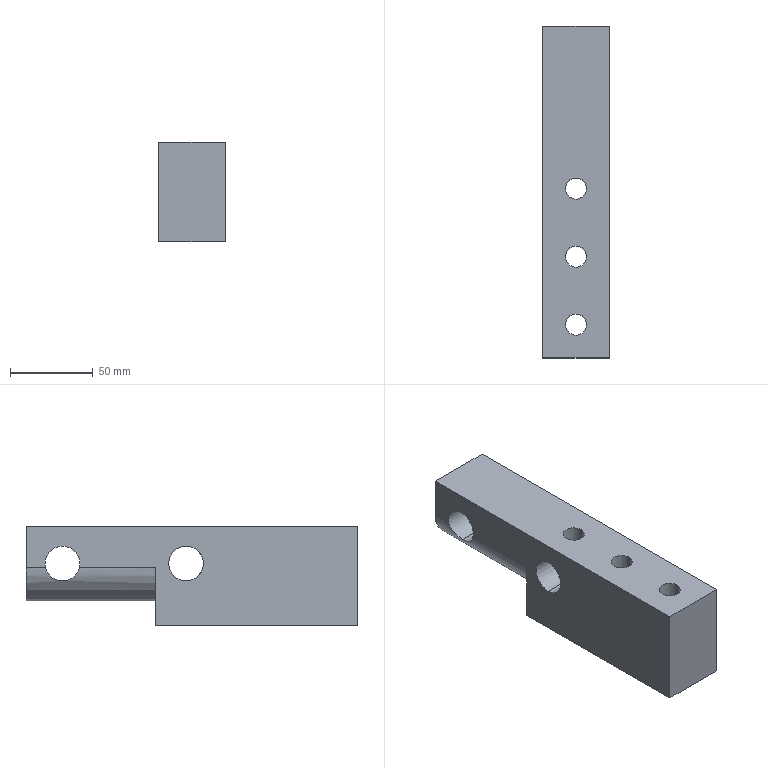Part | SolidWorks | features BaseBody 1 | 1 solid | 20 faces | box 40 x 200 x 60 mm | volume 371568 mm3 | cylinder 13 | plane 7 | commonest cylinder face diameters 12.8 x8 21 x4 40 x1
STEP:
#1=CARTESIAN_POINT('',(20.,67.862,5.));
#2=VERTEX_POINT('',#1);
#3=CARTESIAN_POINT('',(18.33,78.06,-3.));
#4=VERTEX_POINT('',#3);
#5=CARTESIAN_POINT('',(20.,67.862,5.));
#6=CARTESIAN_POINT('',(20.,68.003,4.424));
#7=CARTESIAN_POINT('',(19.975,68.191,3.869));
#8=CARTESIAN_POINT('',(19.886,68.653,2.8));
#9=CARTESIAN_POINT('',(19.821,68.929,2.283));
#10=CARTESIAN_POINT('',(19.661,69.566,1.299));
#11=CARTESIAN_POINT('',(19.568,69.921,0.8415));
#12=CARTESIAN_POINT('',(19.417,70.504,0.2031));
#13=CARTESIAN_POINT('',(19.366,70.708,-0.001681));
#14=CARTESIAN_POINT('',(19.26,71.132,-0.3951));
#15=CARTESIAN_POINT('',(19.205,71.354,-0.5846));
#16=CARTESIAN_POINT('',(19.044,72.039,-1.122));
#17=CARTESIAN_POINT('',(18.938,72.52,-1.438));
#18=CARTESIAN_POINT('',(18.79,73.278,-1.852));
#19=CARTESIAN_POINT('',(18.743,73.537,-1.98));
#20=CARTESIAN_POINT('',(18.653,74.068,-2.216));
#21=CARTESIAN_POINT('',(18.611,74.341,-2.324));
#22=CARTESIAN_POINT('',(18.496,75.171,-2.612));
#23=CARTESIAN_POINT('',(18.435,75.735,-2.756));
#24=CARTESIAN_POINT('',(18.352,76.882,-2.95));
#25=CARTESIAN_POINT('',(18.33,77.468,-3.));
#26=CARTESIAN_POINT('',(18.33,78.06,-3.));
#27=B_SPLINE_CURVE_WITH_KNOTS('',3,(#5,#6,#7,#8,#9,#10,#11,#12,#13,#14,#15,#16,#17,#18,#19,#20,#21,#22,#23,#24,#25,#26),.UNSPECIFIED.,.F.,.F.,(4,2,2,2,2,2,2,2,2,2,4),(0.,0.001752,0.003505,0.005257,0.006134,0.00701,0.008762,0.009639,0.01051,0.01227,0.01402),.UNSPECIFIED.);
#28=EDGE_CURVE('',#2,#4,#27,.T.);
#29=ORIENTED_EDGE('',*,*,#28,.T.);
#30=CARTESIAN_POINT('',(-18.33,78.06,-3.));
#31=VERTEX_POINT('',#30);
#32=CARTESIAN_POINT('',(58.,78.06,-3.));
#33=DIRECTION('',(-1.,0.,0.));
#34=VECTOR('',#33,1000.);
#35=LINE('',#32,#34);
#36=EDGE_CURVE('',#4,#31,#35,.T.);
#37=ORIENTED_EDGE('',*,*,#36,.T.);
#38=CARTESIAN_POINT('',(-20.,67.862,5.));
#39=VERTEX_POINT('',#38);
#40=CARTESIAN_POINT('',(-18.33,78.06,-3.));
#41=CARTESIAN_POINT('',(-18.33,77.469,-3.));
#42=CARTESIAN_POINT('',(-18.352,76.886,-2.95));
#43=CARTESIAN_POINT('',(-18.414,76.024,-2.805));
#44=CARTESIAN_POINT('',(-18.44,75.739,-2.744));
#45=CARTESIAN_POINT('',(-18.5,75.173,-2.6));
#46=CARTESIAN_POINT('',(-18.535,74.891,-2.515));
#47=CARTESIAN_POINT('',(-18.65,74.062,-2.227));
#48=CARTESIAN_POINT('',(-18.74,73.534,-1.992));
#49=CARTESIAN_POINT('',(-18.888,72.774,-1.577));
#50=CARTESIAN_POINT('',(-18.94,72.526,-1.428));
#51=CARTESIAN_POINT('',(-19.045,72.042,-1.109));
#52=CARTESIAN_POINT('',(-19.099,71.805,-0.9388));
#53=CARTESIAN_POINT('',(-19.26,71.123,-0.4035));
#54=CARTESIAN_POINT('',(-19.367,70.702,-0.01284));
#55=CARTESIAN_POINT('',(-19.517,70.119,0.6246));
#56=CARTESIAN_POINT('',(-19.565,69.933,0.8457));
#57=CARTESIAN_POINT('',(-19.657,69.577,1.306));
#58=CARTESIAN_POINT('',(-19.701,69.407,1.545));
#59=CARTESIAN_POINT('',(-19.82,68.931,2.279));
#60=CARTESIAN_POINT('',(-19.885,68.657,2.791));
#61=CARTESIAN_POINT('',(-19.975,68.193,3.862));
#62=CARTESIAN_POINT('',(-20.,68.003,4.424));
#63=CARTESIAN_POINT('',(-20.,67.862,5.));
#64=B_SPLINE_CURVE_WITH_KNOTS('',3,(#40,#41,#42,#43,#44,#45,#46,#47,#48,#49,#50,#51,#52,#53,#54,#55,#56,#57,#58,#59,#60,#61,#62,#63),.UNSPECIFIED.,.F.,.F.,(4,2,2,2,2,2,2,2,2,2,2,4),(0.01402,0.01577,0.01665,0.01752,0.01927,0.02015,0.02102,0.02277,0.02365,0.02452,0.02627,0.02802),.UNSPECIFIED.);
#65=EDGE_CURVE('',#31,#39,#64,.T.);
#66=ORIENTED_EDGE('',*,*,#65,.T.);
#67=CARTESIAN_POINT('',(-20.,78.06,18.));
#68=VERTEX_POINT('',#67);
#69=CARTESIAN_POINT('',(-20.,78.06,7.5));
#70=DIRECTION('',(-1.,0.,0.));
#71=DIRECTION('',(0.,0.,1.));
#72=AXIS2_PLACEMENT_3D('',#69,#70,#71);
#73=CIRCLE('',#72,10.5);
#74=EDGE_CURVE('',#39,#68,#73,.T.);
#75=ORIENTED_EDGE('',*,*,#74,.T.);
#76=CARTESIAN_POINT('',(20.,78.06,18.));
#77=VERTEX_POINT('',#76);
#78=CARTESIAN_POINT('',(58.,78.06,18.));
#79=DIRECTION('',(-1.,0.,0.));
#80=VECTOR('',#79,1000.);
#81=LINE('',#78,#80);
#82=EDGE_CURVE('',#77,#68,#81,.T.);
#83=ORIENTED_EDGE('',*,*,#82,.F.);
#84=CARTESIAN_POINT('',(20.,78.06,7.5));
#85=DIRECTION('',(-1.,0.,0.));
#86=DIRECTION('',(0.,0.,1.));
#87=AXIS2_PLACEMENT_3D('',#84,#85,#86);
#88=CIRCLE('',#87,10.5);
#89=EDGE_CURVE('',#2,#77,#88,.T.);
#90=ORIENTED_EDGE('',*,*,#89,.F.);
#91=EDGE_LOOP('',(#29,#37,#66,#75,#83,#90));
#92=FACE_OUTER_BOUND('',#91,.T.);
#93=CARTESIAN_POINT('',(58.,78.06,7.5));
#94=DIRECTION('',(-1.,0.,0.));
#95=DIRECTION('',(0.,0.,1.));
#96=AXIS2_PLACEMENT_3D('',#93,#94,#95);
#97=CYLINDRICAL_SURFACE('',#96,10.5);
#98=ADVANCED_FACE('',(#92),#97,.F.);
#99=CARTESIAN_POINT('',(20.,3.56,-3.));
#100=VERTEX_POINT('',#99);
#101=CARTESIAN_POINT('',(20.,3.56,18.));
#102=VERTEX_POINT('',#101);
#103=CARTESIAN_POINT('',(20.,3.56,7.5));
#104=DIRECTION('',(-1.,0.,0.));
#105=DIRECTION('',(0.,0.,1.));
#106=AXIS2_PLACEMENT_3D('',#103,#104,#105);
#107=CIRCLE('',#106,10.5);
#108=EDGE_CURVE('',#100,#102,#107,.T.);
#109=ORIENTED_EDGE('',*,*,#108,.F.);
#110=CARTESIAN_POINT('',(6.207,3.56,-3.));
#111=VERTEX_POINT('',#110);
#112=CARTESIAN_POINT('',(58.,3.56,-3.));
#113=DIRECTION('',(-1.,0.,0.));
#114=VECTOR('',#113,1000.);
#115=LINE('',#112,#114);
#116=EDGE_CURVE('',#100,#111,#115,.T.);
#117=ORIENTED_EDGE('',*,*,#116,.T.);
#118=CARTESIAN_POINT('',(6.4,2.,-2.883));
#119=VERTEX_POINT('',#118);
#120=CARTESIAN_POINT('',(6.4,2.,-2.883));
#121=CARTESIAN_POINT('',(6.4,2.259,-2.922));
#122=CARTESIAN_POINT('',(6.384,2.519,-2.952));
#123=CARTESIAN_POINT('',(6.32,3.04,-2.99));
#124=CARTESIAN_POINT('',(6.271,3.304,-3.));
#125=CARTESIAN_POINT('',(6.207,3.56,-3.));
#126=B_SPLINE_CURVE_WITH_KNOTS('',3,(#120,#121,#122,#123,#124,#125),.UNSPECIFIED.,.F.,.F.,(4,2,4),(0.02134,0.02212,0.02291),.UNSPECIFIED.);
#127=EDGE_CURVE('',#119,#111,#126,.T.);
#128=ORIENTED_EDGE('',*,*,#127,.F.);
#129=CARTESIAN_POINT('',(-6.4,2.,-2.883));
#130=VERTEX_POINT('',#129);
#131=CARTESIAN_POINT('',(-6.4,2.,-2.883));
#132=CARTESIAN_POINT('',(-6.4,1.553,-2.816));
#133=CARTESIAN_POINT('',(-6.354,1.12,-2.722));
#134=CARTESIAN_POINT('',(-6.18,0.2803,-2.484));
#135=CARTESIAN_POINT('',(-6.049,-0.1306,-2.339));
#136=CARTESIAN_POINT('',(-5.722,-0.897,-2.016));
#137=CARTESIAN_POINT('',(-5.525,-1.256,-1.839));
#138=CARTESIAN_POINT('',(-5.067,-1.93,-1.459));
#139=CARTESIAN_POINT('',(-4.811,-2.24,-1.26));
#140=CARTESIAN_POINT('',(-4.388,-2.663,-0.9592));
#141=CARTESIAN_POINT('',(-4.241,-2.797,-0.8585));
#142=CARTESIAN_POINT('',(-3.933,-3.053,-0.6579));
#143=CARTESIAN_POINT('',(-3.772,-3.174,-0.5574));
#144=CARTESIAN_POINT('',(-3.272,-3.515,-0.2639));
#145=CARTESIAN_POINT('',(-2.917,-3.712,-0.07815));
#146=CARTESIAN_POINT('',(-2.155,-4.04,0.2517));
#147=CARTESIAN_POINT('',(-1.744,-4.173,0.3961));
#148=CARTESIAN_POINT('',(-1.105,-4.308,0.5463));
#149=CARTESIAN_POINT('',(-0.8875,-4.342,0.5857));
#150=CARTESIAN_POINT('',(-0.4424,-4.389,0.6392));
#151=CARTESIAN_POINT('',(-0.2165,-4.4,0.6528));
#152=CARTESIAN_POINT('',(0.2295,-4.4,0.6522));
#153=CARTESIAN_POINT('',(0.4515,-4.388,0.6384));
#154=CARTESIAN_POINT('',(0.8932,-4.341,0.5847));
#155=CARTESIAN_POINT('',(1.115,-4.306,0.5444));
#156=CARTESIAN_POINT('',(1.756,-4.17,0.3926));
#157=CARTESIAN_POINT('',(2.158,-4.04,0.2509));
#158=CARTESIAN_POINT('',(2.925,-3.708,-0.08206));
#159=CARTESIAN_POINT('',(3.281,-3.509,-0.2694));
#160=CARTESIAN_POINT('',(3.942,-3.058,-0.6575));
#161=CARTESIAN_POINT('',(4.249,-2.803,-0.8599));
#162=CARTESIAN_POINT('',(4.816,-2.234,-1.264));
#163=CARTESIAN_POINT('',(5.07,-1.926,-1.461));
#164=CARTESIAN_POINT('',(5.41,-1.426,-1.743));
#165=CARTESIAN_POINT('',(5.515,-1.253,-1.834));
#166=CARTESIAN_POINT('',(5.712,-0.893,-2.011));
#167=CARTESIAN_POINT('',(5.804,-0.705,-2.097));
#168=CARTESIAN_POINT('',(6.051,-0.1275,-2.34));
#169=CARTESIAN_POINT('',(6.178,0.2748,-2.482));
#170=CARTESIAN_POINT('',(6.31,0.907,-2.662));
#171=CARTESIAN_POINT('',(6.344,1.124,-2.716));
#172=CARTESIAN_POINT('',(6.389,1.561,-2.81));
#173=CARTESIAN_POINT('',(6.4,1.78,-2.85));
#174=CARTESIAN_POINT('',(6.4,2.,-2.883));
#175=B_SPLINE_CURVE_WITH_KNOTS('',3,(#131,#132,#133,#134,#135,#136,#137,#138,#139,#140,#141,#142,#143,#144,#145,#146,#147,#148,#149,#150,#151,#152,#153,#154,#155,#156,#157,#158,#159,#160,#161,#162,#163,#164,#165,#166,#167,#168,#169,#170,#171,#172,#173,#174),.UNSPECIFIED.,.F.,.F.,(4,2,2,2,2,2,2,2,2,2,2,2,2,2,2,2,2,2,2,2,2,4),(0.,0.001334,0.002667,0.004001,0.005334,0.006001,0.006668,0.008001,0.009335,0.01,0.01067,0.01134,0.012,0.01334,0.01467,0.016,0.01734,0.018,0.01867,0.02,0.02067,0.02134),.UNSPECIFIED.);
#176=EDGE_CURVE('',#130,#119,#175,.T.);
#177=ORIENTED_EDGE('',*,*,#176,.F.);
#178=CARTESIAN_POINT('',(-6.207,3.56,-3.));
#179=VERTEX_POINT('',#178);
#180=CARTESIAN_POINT('',(-6.207,3.56,-3.));
#181=CARTESIAN_POINT('',(-6.271,3.307,-3.));
#182=CARTESIAN_POINT('',(-6.319,3.05,-2.991));
#183=CARTESIAN_POINT('',(-6.384,2.528,-2.952));
#184=CARTESIAN_POINT('',(-6.4,2.263,-2.923));
#185=CARTESIAN_POINT('',(-6.4,2.,-2.883));
#186=B_SPLINE_CURVE_WITH_KNOTS('',3,(#180,#181,#182,#183,#184,#185),.UNSPECIFIED.,.F.,.F.,(4,2,4),(0.03996,0.04074,0.04152),.UNSPECIFIED.);
#187=EDGE_CURVE('',#179,#130,#186,.T.);
#188=ORIENTED_EDGE('',*,*,#187,.F.);
#189=CARTESIAN_POINT('',(-20.,3.56,-3.));
#190=VERTEX_POINT('',#189);
#191=CARTESIAN_POINT('',(58.,3.56,-3.));
#192=DIRECTION('',(-1.,0.,0.));
#193=VECTOR('',#192,1000.);
#194=LINE('',#191,#193);
#195=EDGE_CURVE('',#179,#190,#194,.T.);
#196=ORIENTED_EDGE('',*,*,#195,.T.);
#197=CARTESIAN_POINT('',(-20.,3.56,18.));
#198=VERTEX_POINT('',#197);
#199=CARTESIAN_POINT('',(-20.,3.56,7.5));
#200=DIRECTION('',(-1.,0.,0.));
#201=DIRECTION('',(0.,0.,1.));
#202=AXIS2_PLACEMENT_3D('',#199,#200,#201);
#203=CIRCLE('',#202,10.5);
#204=EDGE_CURVE('',#190,#198,#203,.T.);
#205=ORIENTED_EDGE('',*,*,#204,.T.);
#206=CARTESIAN_POINT('',(-6.207,3.56,18.));
#207=VERTEX_POINT('',#206);
#208=CARTESIAN_POINT('',(58.,3.56,18.));
#209=DIRECTION('',(-1.,0.,0.));
#210=VECTOR('',#209,1000.);
#211=LINE('',#208,#210);
#212=EDGE_CURVE('',#207,#198,#211,.T.);
#213=ORIENTED_EDGE('',*,*,#212,.F.);
#214=CARTESIAN_POINT('',(-6.4,2.,17.883));
#215=VERTEX_POINT('',#214);
#216=CARTESIAN_POINT('',(-6.4,2.,17.883));
#217=CARTESIAN_POINT('',(-6.4,2.264,17.923));
#218=CARTESIAN_POINT('',(-6.384,2.525,17.952));
#219=CARTESIAN_POINT('',(-6.319,3.045,17.991));
#220=CARTESIAN_POINT('',(-6.271,3.304,18.));
#221=CARTESIAN_POINT('',(-6.207,3.56,18.));
#222=B_SPLINE_CURVE_WITH_KNOTS('',3,(#216,#217,#218,#219,#220,#221),.UNSPECIFIED.,.F.,.F.,(4,2,4),(0.,0.0007878,0.001576),.UNSPECIFIED.);
#223=EDGE_CURVE('',#215,#207,#222,.T.);
#224=ORIENTED_EDGE('',*,*,#223,.F.);
#225=CARTESIAN_POINT('',(6.4,2.,17.883));
#226=VERTEX_POINT('',#225);
#227=CARTESIAN_POINT('',(6.4,2.,17.883));
#228=CARTESIAN_POINT('',(6.4,1.778,17.85));
#229=CARTESIAN_POINT('',(6.388,1.556,17.809));
#230=CARTESIAN_POINT('',(6.343,1.121,17.715));
#231=CARTESIAN_POINT('',(6.31,0.9071,17.662));
#232=CARTESIAN_POINT('',(6.178,0.2763,17.483));
#233=CARTESIAN_POINT('',(6.048,-0.134,17.338));
#234=CARTESIAN_POINT('',(5.72,-0.9001,17.015));
#235=CARTESIAN_POINT('',(5.523,-1.259,16.837));
#236=CARTESIAN_POINT('',(5.065,-1.933,16.457));
#237=CARTESIAN_POINT('',(4.809,-2.242,16.258));
#238=CARTESIAN_POINT('',(4.387,-2.664,15.958));
#239=CARTESIAN_POINT('',(4.24,-2.798,15.857));
#240=CARTESIAN_POINT('',(3.932,-3.054,15.657));
#241=CARTESIAN_POINT('',(3.77,-3.176,15.556));
#242=CARTESIAN_POINT('',(3.27,-3.516,15.263));
#243=CARTESIAN_POINT('',(2.916,-3.712,15.078));
#244=CARTESIAN_POINT('',(2.155,-4.041,14.748));
#245=CARTESIAN_POINT('',(1.743,-4.173,14.604));
#246=CARTESIAN_POINT('',(1.105,-4.308,14.454));
#247=CARTESIAN_POINT('',(0.8875,-4.342,14.414));
#248=CARTESIAN_POINT('',(0.4424,-4.389,14.361));
#249=CARTESIAN_POINT('',(0.217,-4.4,14.347));
#250=CARTESIAN_POINT('',(-0.2285,-4.4,14.348));
#251=CARTESIAN_POINT('',(-0.4503,-4.388,14.362));
#252=CARTESIAN_POINT('',(-0.892,-4.341,14.415));
#253=CARTESIAN_POINT('',(-1.113,-4.306,14.455));
#254=CARTESIAN_POINT('',(-1.754,-4.171,14.607));
#255=CARTESIAN_POINT('',(-2.156,-4.04,14.748));
#256=CARTESIAN_POINT('',(-2.924,-3.708,15.081));
#257=CARTESIAN_POINT('',(-3.279,-3.511,15.268));
#258=CARTESIAN_POINT('',(-3.939,-3.06,15.656));
#259=CARTESIAN_POINT('',(-4.247,-2.804,15.859));
#260=CARTESIAN_POINT('',(-4.814,-2.237,16.262));
#261=CARTESIAN_POINT('',(-5.068,-1.929,16.459));
#262=CARTESIAN_POINT('',(-5.407,-1.43,16.741));
#263=CARTESIAN_POINT('',(-5.513,-1.257,16.832));
#264=CARTESIAN_POINT('',(-5.71,-0.8971,17.009));
#265=CARTESIAN_POINT('',(-5.802,-0.7091,17.095));
#266=CARTESIAN_POINT('',(-6.049,-0.1327,17.338));
#267=CARTESIAN_POINT('',(-6.176,0.2691,17.481));
#268=CARTESIAN_POINT('',(-6.353,1.112,17.72));
#269=CARTESIAN_POINT('',(-6.4,1.554,17.816));
#270=CARTESIAN_POINT('',(-6.4,2.,17.883));
#271=B_SPLINE_CURVE_WITH_KNOTS('',3,(#227,#228,#229,#230,#231,#232,#233,#234,#235,#236,#237,#238,#239,#240,#241,#242,#243,#244,#245,#246,#247,#248,#249,#250,#251,#252,#253,#254,#255,#256,#257,#258,#259,#260,#261,#262,#263,#264,#265,#266,#267,#268,#269,#270),.UNSPECIFIED.,.F.,.F.,(4,2,2,2,2,2,2,2,2,2,2,2,2,2,2,2,2,2,2,2,2,4),(0.02022,0.02089,0.02156,0.02289,0.02422,0.02555,0.02622,0.02689,0.02822,0.02955,0.03022,0.03089,0.03155,0.03222,0.03355,0.03488,0.03622,0.03755,0.03822,0.03888,0.04022,0.04155),.UNSPECIFIED.);
#272=EDGE_CURVE('',#226,#215,#271,.T.);
#273=ORIENTED_EDGE('',*,*,#272,.F.);
#274=CARTESIAN_POINT('',(6.207,3.56,18.));
#275=VERTEX_POINT('',#274);
#276=CARTESIAN_POINT('',(6.207,3.56,18.));
#277=CARTESIAN_POINT('',(6.272,3.302,18.));
#278=CARTESIAN_POINT('',(6.32,3.043,17.991));
#279=CARTESIAN_POINT('',(6.384,2.523,17.952));
#280=CARTESIAN_POINT('',(6.4,2.262,17.923));
#281=CARTESIAN_POINT('',(6.4,2.,17.883));
#282=B_SPLINE_CURVE_WITH_KNOTS('',3,(#276,#277,#278,#279,#280,#281),.UNSPECIFIED.,.F.,.F.,(4,2,4),(0.01865,0.01943,0.02022),.UNSPECIFIED.);
#283=EDGE_CURVE('',#275,#226,#282,.T.);
#284=ORIENTED_EDGE('',*,*,#283,.F.);
#285=CARTESIAN_POINT('',(58.,3.56,18.));
#286=DIRECTION('',(-1.,0.,0.));
#287=VECTOR('',#286,1000.);
#288=LINE('',#285,#287);
#289=EDGE_CURVE('',#102,#275,#288,.T.);
#290=ORIENTED_EDGE('',*,*,#289,.F.);
#291=EDGE_LOOP('',(#109,#117,#128,#177,#188,#196,#205,#213,#224,#273,#284,#290));
#292=FACE_OUTER_BOUND('',#291,.T.);
#293=CARTESIAN_POINT('',(58.,3.56,7.5));
#294=DIRECTION('',(-1.,0.,0.));
#295=DIRECTION('',(0.,0.,1.));
#296=AXIS2_PLACEMENT_3D('',#293,#294,#295);
#297=CYLINDRICAL_SURFACE('',#296,10.5);
#298=ADVANCED_FACE('',(#292),#297,.F.);
#299=ORIENTED_EDGE('',*,*,#176,.T.);
#300=CARTESIAN_POINT('',(6.4,2.,-30.));
#301=VERTEX_POINT('',#300);
#302=CARTESIAN_POINT('',(6.4,2.,48.));
#303=DIRECTION('',(0.,0.,-1.));
#304=VECTOR('',#303,1000.);
#305=LINE('',#302,#304);
#306=EDGE_CURVE('',#119,#301,#305,.T.);
#307=ORIENTED_EDGE('',*,*,#306,.T.);
#308=CARTESIAN_POINT('',(-6.4,2.,-30.));
#309=VERTEX_POINT('',#308);
#310=CARTESIAN_POINT('',(0.,2.,-30.));
#311=DIRECTION('',(0.,0.,-1.));
#312=DIRECTION('',(1.,0.,0.));
#313=AXIS2_PLACEMENT_3D('',#310,#311,#312);
#314=CIRCLE('',#313,6.4);
#315=EDGE_CURVE('',#301,#309,#314,.T.);
#316=ORIENTED_EDGE('',*,*,#315,.T.);
#317=CARTESIAN_POINT('',(-6.4,2.,48.));
#318=DIRECTION('',(0.,0.,-1.));
#319=VECTOR('',#318,1000.);
#320=LINE('',#317,#319);
#321=EDGE_CURVE('',#130,#309,#320,.T.);
#322=ORIENTED_EDGE('',*,*,#321,.F.);
#323=EDGE_LOOP('',(#299,#307,#316,#322));
#324=FACE_OUTER_BOUND('',#323,.T.);
#325=CARTESIAN_POINT('',(0.,2.,48.));
#326=DIRECTION('',(0.,0.,-1.));
#327=DIRECTION('',(-1.,0.,0.));
#328=AXIS2_PLACEMENT_3D('',#325,#326,#327);
#329=CYLINDRICAL_SURFACE('',#328,6.4);
#330=ADVANCED_FACE('',(#324),#329,.F.);
#331=CARTESIAN_POINT('',(6.4,-80.,30.));
#332=VERTEX_POINT('',#331);
#333=CARTESIAN_POINT('',(-6.4,-80.,30.));
#334=VERTEX_POINT('',#333);
#335=CARTESIAN_POINT('',(0.,-80.,30.));
#336=DIRECTION('',(0.,0.,-1.));
#337=DIRECTION('',(-1.,0.,0.));
#338=AXIS2_PLACEMENT_3D('',#335,#336,#337);
#339=CIRCLE('',#338,6.4);
#340=EDGE_CURVE('',#332,#334,#339,.T.);
#341=ORIENTED_EDGE('',*,*,#340,.F.);
#342=CARTESIAN_POINT('',(6.4,-80.,-30.));
#343=VERTEX_POINT('',#342);
#344=CARTESIAN_POINT('',(6.4,-80.,48.));
#345=DIRECTION('',(0.,0.,-1.));
#346=VECTOR('',#345,1000.);
#347=LINE('',#344,#346);
#348=EDGE_CURVE('',#332,#343,#347,.T.);
#349=ORIENTED_EDGE('',*,*,#348,.T.);
#350=CARTESIAN_POINT('',(-6.4,-80.,-30.));
#351=VERTEX_POINT('',#350);
#352=CARTESIAN_POINT('',(0.,-80.,-30.));
#353=DIRECTION('',(0.,0.,-1.));
#354=DIRECTION('',(-1.,0.,0.));
#355=AXIS2_PLACEMENT_3D('',#352,#353,#354);
#356=CIRCLE('',#355,6.4);
#357=EDGE_CURVE('',#343,#351,#356,.T.);
#358=ORIENTED_EDGE('',*,*,#357,.T.);
#359=CARTESIAN_POINT('',(-6.4,-80.,48.));
#360=DIRECTION('',(0.,0.,-1.));
#361=VECTOR('',#360,1000.);
#362=LINE('',#359,#361);
#363=EDGE_CURVE('',#334,#351,#362,.T.);
#364=ORIENTED_EDGE('',*,*,#363,.F.);
#365=EDGE_LOOP('',(#341,#349,#358,#364));
#366=FACE_OUTER_BOUND('',#365,.T.);
#367=CARTESIAN_POINT('',(0.,-80.,48.));
#368=DIRECTION('',(0.,0.,-1.));
#369=DIRECTION('',(-1.,0.,0.));
#370=AXIS2_PLACEMENT_3D('',#367,#368,#369);
#371=CYLINDRICAL_SURFACE('',#370,6.4);
#372=ADVANCED_FACE('',(#366),#371,.F.);
#373=CARTESIAN_POINT('',(6.4,-39.,30.));
#374=VERTEX_POINT('',#373);
#375=CARTESIAN_POINT('',(-6.4,-39.,30.));
#376=VERTEX_POINT('',#375);
#377=CARTESIAN_POINT('',(0.,-39.,30.));
#378=DIRECTION('',(0.,0.,-1.));
#379=DIRECTION('',(-1.,0.,0.));
#380=AXIS2_PLACEMENT_3D('',#377,#378,#379);
#381=CIRCLE('',#380,6.4);
#382=EDGE_CURVE('',#374,#376,#381,.T.);
#383=ORIENTED_EDGE('',*,*,#382,.F.);
#384=CARTESIAN_POINT('',(6.4,-39.,-30.));
#385=VERTEX_POINT('',#384);
#386=CARTESIAN_POINT('',(6.4,-39.,48.));
#387=DIRECTION('',(0.,0.,-1.));
#388=VECTOR('',#387,1000.);
#389=LINE('',#386,#388);
#390=EDGE_CURVE('',#374,#385,#389,.T.);
#391=ORIENTED_EDGE('',*,*,#390,.T.);
#392=CARTESIAN_POINT('',(-6.4,-39.,-30.));
#393=VERTEX_POINT('',#392);
#394=CARTESIAN_POINT('',(0.,-39.,-30.));
#395=DIRECTION('',(0.,0.,-1.));
#396=DIRECTION('',(-1.,0.,0.));
#397=AXIS2_PLACEMENT_3D('',#394,#395,#396);
#398=CIRCLE('',#397,6.4);
#399=EDGE_CURVE('',#385,#393,#398,.T.);
#400=ORIENTED_EDGE('',*,*,#399,.T.);
#401=CARTESIAN_POINT('',(-6.4,-39.,48.));
#402=DIRECTION('',(0.,0.,-1.));
#403=VECTOR('',#402,1000.);
#404=LINE('',#401,#403);
#405=EDGE_CURVE('',#376,#393,#404,.T.);
#406=ORIENTED_EDGE('',*,*,#405,.F.);
#407=EDGE_LOOP('',(#383,#391,#400,#406));
#408=FACE_OUTER_BOUND('',#407,.T.);
#409=CARTESIAN_POINT('',(0.,-39.,48.));
#410=DIRECTION('',(0.,0.,-1.));
#411=DIRECTION('',(-1.,0.,0.));
#412=AXIS2_PLACEMENT_3D('',#409,#410,#411);
#413=CYLINDRICAL_SURFACE('',#412,6.4);
#414=ADVANCED_FACE('',(#408),#413,.F.);
#415=CARTESIAN_POINT('',(6.4,2.,30.));
#416=VERTEX_POINT('',#415);
#417=CARTESIAN_POINT('',(-6.4,2.,30.));
#418=VERTEX_POINT('',#417);
#419=CARTESIAN_POINT('',(0.,2.,30.));
#420=DIRECTION('',(0.,0.,-1.));
#421=DIRECTION('',(-1.,0.,0.));
#422=AXIS2_PLACEMENT_3D('',#419,#420,#421);
#423=CIRCLE('',#422,6.4);
#424=EDGE_CURVE('',#416,#418,#423,.T.);
#425=ORIENTED_EDGE('',*,*,#424,.F.);
#426=CARTESIAN_POINT('',(6.4,2.,48.));
#427=DIRECTION('',(0.,0.,-1.));
#428=VECTOR('',#427,1000.);
#429=LINE('',#426,#428);
#430=EDGE_CURVE('',#416,#226,#429,.T.);
#431=ORIENTED_EDGE('',*,*,#430,.T.);
#432=ORIENTED_EDGE('',*,*,#272,.T.);
#433=CARTESIAN_POINT('',(-6.4,2.,48.));
#434=DIRECTION('',(0.,0.,-1.));
#435=VECTOR('',#434,1000.);
#436=LINE('',#433,#435);
#437=EDGE_CURVE('',#418,#215,#436,.T.);
#438=ORIENTED_EDGE('',*,*,#437,.F.);
#439=EDGE_LOOP('',(#425,#431,#432,#438));
#440=FACE_OUTER_BOUND('',#439,.T.);
#441=CARTESIAN_POINT('',(0.,2.,48.));
#442=DIRECTION('',(0.,0.,-1.));
#443=DIRECTION('',(-1.,0.,0.));
#444=AXIS2_PLACEMENT_3D('',#441,#442,#443);
#445=CYLINDRICAL_SURFACE('',#444,6.4);
#446=ADVANCED_FACE('',(#440),#445,.F.);
#447=ORIENTED_EDGE('',*,*,#430,.F.);
#448=CARTESIAN_POINT('',(0.,2.,30.));
#449=DIRECTION('',(0.,0.,-1.));
#450=DIRECTION('',(-1.,0.,0.));
#451=AXIS2_PLACEMENT_3D('',#448,#449,#450);
#452=CIRCLE('',#451,6.4);
#453=EDGE_CURVE('',#418,#416,#452,.T.);
#454=ORIENTED_EDGE('',*,*,#453,.F.);
#455=ORIENTED_EDGE('',*,*,#437,.T.);
#456=ORIENTED_EDGE('',*,*,#223,.T.);
#457=CARTESIAN_POINT('',(-6.207,3.56,18.));
#458=CARTESIAN_POINT('',(-6.163,3.734,18.));
#459=CARTESIAN_POINT('',(-6.112,3.907,17.996));
#460=CARTESIAN_POINT('',(-5.996,4.246,17.979));
#461=CARTESIAN_POINT('',(-5.931,4.412,17.967));
#462=CARTESIAN_POINT('',(-5.716,4.9,17.919));
#463=CARTESIAN_POINT('',(-5.548,5.211,17.874));
#464=CARTESIAN_POINT('',(-4.963,6.103,17.705));
#465=CARTESIAN_POINT('',(-4.486,6.618,17.555));
#466=CARTESIAN_POINT('',(-3.377,7.482,17.251));
#467=CARTESIAN_POINT('',(-2.765,7.816,17.102));
#468=CARTESIAN_POINT('',(-1.419,8.281,16.882));
#469=CARTESIAN_POINT('',(-0.7225,8.4,16.818));
#470=CARTESIAN_POINT('',(0.3589,8.4,16.818));
#471=CARTESIAN_POINT('',(0.7155,8.37,16.834));
#472=CARTESIAN_POINT('',(1.415,8.252,16.894));
#473=CARTESIAN_POINT('',(1.76,8.163,16.938));
#474=CARTESIAN_POINT('',(2.432,7.93,17.048));
#475=CARTESIAN_POINT('',(2.753,7.788,17.113));
#476=CARTESIAN_POINT('',(3.367,7.454,17.253));
#477=CARTESIAN_POINT('',(3.663,7.26,17.329));
#478=CARTESIAN_POINT('',(4.215,6.829,17.481));
#479=CARTESIAN_POINT('',(4.471,6.593,17.556));
#480=CARTESIAN_POINT('',(4.826,6.207,17.662));
#481=CARTESIAN_POINT('',(4.939,6.074,17.696));
#482=CARTESIAN_POINT('',(5.156,5.796,17.76));
#483=CARTESIAN_POINT('',(5.26,5.651,17.791));
#484=CARTESIAN_POINT('',(5.55,5.206,17.875));
#485=CARTESIAN_POINT('',(5.718,4.896,17.92));
#486=CARTESIAN_POINT('',(5.931,4.411,17.967));
#487=CARTESIAN_POINT('',(5.996,4.246,17.979));
#488=CARTESIAN_POINT('',(6.112,3.908,17.996));
#489=CARTESIAN_POINT('',(6.163,3.734,18.));
#490=CARTESIAN_POINT('',(6.207,3.56,18.));
#491=B_SPLINE_CURVE_WITH_KNOTS('',3,(#457,#458,#459,#460,#461,#462,#463,#464,#465,#466,#467,#468,#469,#470,#471,#472,#473,#474,#475,#476,#477,#478,#479,#480,#481,#482,#483,#484,#485,#486,#487,#488,#489,#490),.UNSPECIFIED.,.F.,.F.,(4,2,2,2,2,2,2,2,2,2,2,2,2,2,2,2,4),(0.001576,0.002109,0.002642,0.003709,0.005843,0.007977,0.01011,0.01118,0.01224,0.01331,0.01438,0.01544,0.01598,0.01651,0.01758,0.01811,0.01865),.UNSPECIFIED.);
#492=EDGE_CURVE('',#207,#275,#491,.T.);
#493=ORIENTED_EDGE('',*,*,#492,.T.);
#494=ORIENTED_EDGE('',*,*,#283,.T.);
#495=EDGE_LOOP('',(#447,#454,#455,#456,#493,#494));
#496=FACE_OUTER_BOUND('',#495,.T.);
#497=CARTESIAN_POINT('',(0.,2.,48.));
#498=DIRECTION('',(0.,0.,-1.));
#499=DIRECTION('',(-1.,0.,0.));
#500=AXIS2_PLACEMENT_3D('',#497,#498,#499);
#501=CYLINDRICAL_SURFACE('',#500,6.4);
#502=ADVANCED_FACE('',(#496),#501,.F.);
#503=CARTESIAN_POINT('',(0.,2.,-30.));
#504=DIRECTION('',(0.,0.,-1.));
#505=DIRECTION('',(1.,0.,0.));
#506=AXIS2_PLACEMENT_3D('',#503,#504,#505);
#507=CIRCLE('',#506,6.4);
#508=EDGE_CURVE('',#309,#301,#507,.T.);
#509=ORIENTED_EDGE('',*,*,#508,.F.);
#510=ORIENTED_EDGE('',*,*,#315,.F.);
#511=EDGE_LOOP('',(#509,#510));
#512=FACE_BOUND('',#511,.T.);
#513=CARTESIAN_POINT('',(0.,-80.,-30.));
#514=DIRECTION('',(0.,0.,-1.));
#515=DIRECTION('',(-1.,0.,0.));
#516=AXIS2_PLACEMENT_3D('',#513,#514,#515);
#517=CIRCLE('',#516,6.4);
#518=EDGE_CURVE('',#351,#343,#517,.T.);
#519=ORIENTED_EDGE('',*,*,#518,.F.);
#520=ORIENTED_EDGE('',*,*,#357,.F.);
#521=EDGE_LOOP('',(#519,#520));
#522=FACE_BOUND('',#521,.T.);
#523=CARTESIAN_POINT('',(0.,-39.,-30.));
#524=DIRECTION('',(0.,0.,-1.));
#525=DIRECTION('',(-1.,0.,0.));
#526=AXIS2_PLACEMENT_3D('',#523,#524,#525);
#527=CIRCLE('',#526,6.4);
#528=EDGE_CURVE('',#393,#385,#527,.T.);
#529=ORIENTED_EDGE('',*,*,#528,.F.);
#530=ORIENTED_EDGE('',*,*,#399,.F.);
#531=EDGE_LOOP('',(#529,#530));
#532=FACE_BOUND('',#531,.T.);
#533=CARTESIAN_POINT('',(20.,22.,-30.));
#534=VERTEX_POINT('',#533);
#535=CARTESIAN_POINT('',(-20.,22.,-30.));
#536=VERTEX_POINT('',#535);
#537=CARTESIAN_POINT('',(0.,22.,-30.));
#538=DIRECTION('',(-1.,0.,0.));
#539=VECTOR('',#538,1000.);
#540=LINE('',#537,#539);
#541=EDGE_CURVE('',#534,#536,#540,.T.);
#542=ORIENTED_EDGE('',*,*,#541,.F.);
#543=CARTESIAN_POINT('',(20.,-100.,-30.));
#544=VERTEX_POINT('',#543);
#545=CARTESIAN_POINT('',(20.,100.,-30.));
#546=DIRECTION('',(0.,-1.,0.));
#547=VECTOR('',#546,1000.);
#548=LINE('',#545,#547);
#549=EDGE_CURVE('',#534,#544,#548,.T.);
#550=ORIENTED_EDGE('',*,*,#549,.T.);
#551=CARTESIAN_POINT('',(-20.,-100.,-30.));
#552=VERTEX_POINT('',#551);
#553=CARTESIAN_POINT('',(-20.,-100.,-30.));
#554=DIRECTION('',(-1.,0.,0.));
#555=VECTOR('',#554,1000.);
#556=LINE('',#553,#555);
#557=EDGE_CURVE('',#544,#552,#556,.T.);
#558=ORIENTED_EDGE('',*,*,#557,.T.);
#559=CARTESIAN_POINT('',(-20.,100.,-30.));
#560=DIRECTION('',(0.,-1.,0.));
#561=VECTOR('',#560,1000.);
#562=LINE('',#559,#561);
#563=EDGE_CURVE('',#536,#552,#562,.T.);
#564=ORIENTED_EDGE('',*,*,#563,.F.);
#565=EDGE_LOOP('',(#542,#550,#558,#564));
#566=FACE_OUTER_BOUND('',#565,.T.);
#567=CARTESIAN_POINT('',(-20.,100.,-30.));
#568=DIRECTION('',(0.,0.,1.));
#569=DIRECTION('',(1.,0.,0.));
#570=AXIS2_PLACEMENT_3D('',#567,#568,#569);
#571=PLANE('',#570);
#572=ADVANCED_FACE('',(#512,#522,#532,#566),#571,.F.);
#573=CARTESIAN_POINT('',(-20.,3.56,7.5));
#574=DIRECTION('',(-1.,0.,0.));
#575=DIRECTION('',(0.,0.,1.));
#576=AXIS2_PLACEMENT_3D('',#573,#574,#575);
#577=CIRCLE('',#576,10.5);
#578=EDGE_CURVE('',#198,#190,#577,.T.);
#579=ORIENTED_EDGE('',*,*,#578,.F.);
#580=ORIENTED_EDGE('',*,*,#204,.F.);
#581=EDGE_LOOP('',(#579,#580));
#582=FACE_BOUND('',#581,.T.);
#583=CARTESIAN_POINT('',(-20.,88.258,5.));
#584=VERTEX_POINT('',#583);
#585=CARTESIAN_POINT('',(-20.,100.,5.));
#586=VERTEX_POINT('',#585);
#587=CARTESIAN_POINT('',(-20.,22.,5.));
#588=DIRECTION('',(0.,1.,0.));
#589=VECTOR('',#588,1000.);
#590=LINE('',#587,#589);
#591=EDGE_CURVE('',#584,#586,#590,.T.);
#592=ORIENTED_EDGE('',*,*,#591,.F.);
#593=CARTESIAN_POINT('',(-20.,78.06,7.5));
#594=DIRECTION('',(-1.,0.,0.));
#595=DIRECTION('',(0.,0.,1.));
#596=AXIS2_PLACEMENT_3D('',#593,#594,#595);
#597=CIRCLE('',#596,10.5);
#598=EDGE_CURVE('',#68,#584,#597,.T.);
#599=ORIENTED_EDGE('',*,*,#598,.F.);
#600=ORIENTED_EDGE('',*,*,#74,.F.);
#601=CARTESIAN_POINT('',(-20.,22.,5.));
#602=VERTEX_POINT('',#601);
#603=CARTESIAN_POINT('',(-20.,22.,5.));
#604=DIRECTION('',(0.,1.,0.));
#605=VECTOR('',#604,1000.);
#606=LINE('',#603,#605);
#607=EDGE_CURVE('',#602,#39,#606,.T.);
#608=ORIENTED_EDGE('',*,*,#607,.F.);
#609=CARTESIAN_POINT('',(-20.,22.,0.));
#610=DIRECTION('',(0.,0.,1.));
#611=VECTOR('',#610,1000.);
#612=LINE('',#609,#611);
#613=EDGE_CURVE('',#536,#602,#612,.T.);
#614=ORIENTED_EDGE('',*,*,#613,.F.);
#615=ORIENTED_EDGE('',*,*,#563,.T.);
#616=CARTESIAN_POINT('',(-20.,-100.,30.));
#617=VERTEX_POINT('',#616);
#618=CARTESIAN_POINT('',(-20.,-100.,-30.));
#619=DIRECTION('',(0.,0.,1.));
#620=VECTOR('',#619,1000.);
#621=LINE('',#618,#620);
#622=EDGE_CURVE('',#552,#617,#621,.T.);
#623=ORIENTED_EDGE('',*,*,#622,.T.);
#624=CARTESIAN_POINT('',(-20.,100.,30.));
#625=VERTEX_POINT('',#624);
#626=CARTESIAN_POINT('',(-20.,100.,30.));
#627=DIRECTION('',(0.,-1.,0.));
#628=VECTOR('',#627,1000.);
#629=LINE('',#626,#628);
#630=EDGE_CURVE('',#625,#617,#629,.T.);
#631=ORIENTED_EDGE('',*,*,#630,.F.);
#632=CARTESIAN_POINT('',(-20.,100.,-30.));
#633=DIRECTION('',(0.,0.,1.));
#634=VECTOR('',#633,1000.);
#635=LINE('',#632,#634);
#636=EDGE_CURVE('',#586,#625,#635,.T.);
#637=ORIENTED_EDGE('',*,*,#636,.F.);
#638=EDGE_LOOP('',(#592,#599,#600,#608,#614,#615,#623,#631,#637));
#639=FACE_OUTER_BOUND('',#638,.T.);
#640=CARTESIAN_POINT('',(-20.,100.,-30.));
#641=DIRECTION('',(1.,0.,0.));
#642=DIRECTION('',(0.,0.,-1.));
#643=AXIS2_PLACEMENT_3D('',#640,#641,#642);
#644=PLANE('',#643);
#645=ADVANCED_FACE('',(#582,#639),#644,.F.);
#646=CARTESIAN_POINT('',(20.,100.,30.));
#647=VERTEX_POINT('',#646);
#648=CARTESIAN_POINT('',(20.,100.,5.));
#649=VERTEX_POINT('',#648);
#650=CARTESIAN_POINT('',(20.,100.,-30.));
#651=DIRECTION('',(0.,0.,-1.));
#652=VECTOR('',#651,1000.);
#653=LINE('',#650,#652);
#654=EDGE_CURVE('',#647,#649,#653,.T.);
#655=ORIENTED_EDGE('',*,*,#654,.T.);
#656=CARTESIAN_POINT('',(0.,100.,5.));
#657=DIRECTION('',(0.,1.,0.));
#658=DIRECTION('',(0.,0.,1.));
#659=AXIS2_PLACEMENT_3D('',#656,#657,#658);
#660=CIRCLE('',#659,20.);
#661=EDGE_CURVE('',#649,#586,#660,.T.);
#662=ORIENTED_EDGE('',*,*,#661,.T.);
#663=ORIENTED_EDGE('',*,*,#636,.T.);
#664=CARTESIAN_POINT('',(-20.,100.,30.));
#665=DIRECTION('',(1.,0.,0.));
#666=VECTOR('',#665,1000.);
#667=LINE('',#664,#666);
#668=EDGE_CURVE('',#625,#647,#667,.T.);
#669=ORIENTED_EDGE('',*,*,#668,.T.);
#670=EDGE_LOOP('',(#655,#662,#663,#669));
#671=FACE_OUTER_BOUND('',#670,.T.);
#672=CARTESIAN_POINT('',(0.,100.,0.));
#673=DIRECTION('',(0.,1.,0.));
#674=DIRECTION('',(0.,0.,1.));
#675=AXIS2_PLACEMENT_3D('',#672,#673,#674);
#676=PLANE('',#675);
#677=ADVANCED_FACE('',(#671),#676,.T.);
#678=CARTESIAN_POINT('',(20.,3.56,7.5));
#679=DIRECTION('',(-1.,0.,0.));
#680=DIRECTION('',(0.,0.,1.));
#681=AXIS2_PLACEMENT_3D('',#678,#679,#680);
#682=CIRCLE('',#681,10.5);
#683=EDGE_CURVE('',#102,#100,#682,.T.);
#684=ORIENTED_EDGE('',*,*,#683,.T.);
#685=ORIENTED_EDGE('',*,*,#108,.T.);
#686=EDGE_LOOP('',(#684,#685));
#687=FACE_BOUND('',#686,.T.);
#688=CARTESIAN_POINT('',(20.,22.,5.));
#689=VERTEX_POINT('',#688);
#690=CARTESIAN_POINT('',(20.,22.,5.));
#691=DIRECTION('',(0.,1.,0.));
#692=VECTOR('',#691,1000.);
#693=LINE('',#690,#692);
#694=EDGE_CURVE('',#689,#2,#693,.T.);
#695=ORIENTED_EDGE('',*,*,#694,.T.);
#696=ORIENTED_EDGE('',*,*,#89,.T.);
#697=CARTESIAN_POINT('',(20.,88.258,5.));
#698=VERTEX_POINT('',#697);
#699=CARTESIAN_POINT('',(20.,78.06,7.5));
#700=DIRECTION('',(-1.,0.,0.));
#701=DIRECTION('',(0.,0.,1.));
#702=AXIS2_PLACEMENT_3D('',#699,#700,#701);
#703=CIRCLE('',#702,10.5);
#704=EDGE_CURVE('',#77,#698,#703,.T.);
#705=ORIENTED_EDGE('',*,*,#704,.T.);
#706=CARTESIAN_POINT('',(20.,22.,5.));
#707=DIRECTION('',(0.,1.,0.));
#708=VECTOR('',#707,1000.);
#709=LINE('',#706,#708);
#710=EDGE_CURVE('',#698,#649,#709,.T.);
#711=ORIENTED_EDGE('',*,*,#710,.T.);
#712=ORIENTED_EDGE('',*,*,#654,.F.);
#713=CARTESIAN_POINT('',(20.,-100.,30.));
#714=VERTEX_POINT('',#713);
#715=CARTESIAN_POINT('',(20.,100.,30.));
#716=DIRECTION('',(0.,-1.,0.));
#717=VECTOR('',#716,1000.);
#718=LINE('',#715,#717);
#719=EDGE_CURVE('',#647,#714,#718,.T.);
#720=ORIENTED_EDGE('',*,*,#719,.T.);
#721=CARTESIAN_POINT('',(20.,-100.,-30.));
#722=DIRECTION('',(0.,0.,-1.));
#723=VECTOR('',#722,1000.);
#724=LINE('',#721,#723);
#725=EDGE_CURVE('',#714,#544,#724,.T.);
#726=ORIENTED_EDGE('',*,*,#725,.T.);
#727=ORIENTED_EDGE('',*,*,#549,.F.);
#728=CARTESIAN_POINT('',(20.,22.,0.));
#729=DIRECTION('',(0.,0.,-1.));
#730=VECTOR('',#729,1000.);
#731=LINE('',#728,#730);
#732=EDGE_CURVE('',#689,#534,#731,.T.);
#733=ORIENTED_EDGE('',*,*,#732,.F.);
#734=EDGE_LOOP('',(#695,#696,#705,#711,#712,#720,#726,#727,#733));
#735=FACE_OUTER_BOUND('',#734,.T.);
#736=CARTESIAN_POINT('',(20.,100.,-30.));
#737=DIRECTION('',(-1.,0.,0.));
#738=DIRECTION('',(0.,0.,1.));
#739=AXIS2_PLACEMENT_3D('',#736,#737,#738);
#740=PLANE('',#739);
#741=ADVANCED_FACE('',(#687,#735),#740,.F.);
#742=ORIENTED_EDGE('',*,*,#453,.T.);
#743=ORIENTED_EDGE('',*,*,#424,.T.);
#744=EDGE_LOOP('',(#742,#743));
#745=FACE_BOUND('',#744,.T.);
#746=CARTESIAN_POINT('',(0.,-80.,30.));
#747=DIRECTION('',(0.,0.,-1.));
#748=DIRECTION('',(-1.,0.,0.));
#749=AXIS2_PLACEMENT_3D('',#746,#747,#748);
#750=CIRCLE('',#749,6.4);
#751=EDGE_CURVE('',#334,#332,#750,.T.);
#752=ORIENTED_EDGE('',*,*,#751,.T.);
#753=ORIENTED_EDGE('',*,*,#340,.T.);
#754=EDGE_LOOP('',(#752,#753));
#755=FACE_BOUND('',#754,.T.);
#756=CARTESIAN_POINT('',(0.,-39.,30.));
#757=DIRECTION('',(0.,0.,-1.));
#758=DIRECTION('',(-1.,0.,0.));
#759=AXIS2_PLACEMENT_3D('',#756,#757,#758);
#760=CIRCLE('',#759,6.4);
#761=EDGE_CURVE('',#376,#374,#760,.T.);
#762=ORIENTED_EDGE('',*,*,#761,.T.);
#763=ORIENTED_EDGE('',*,*,#382,.T.);
#764=EDGE_LOOP('',(#762,#763));
#765=FACE_BOUND('',#764,.T.);
#766=CARTESIAN_POINT('',(-20.,-100.,30.));
#767=DIRECTION('',(1.,0.,0.));
#768=VECTOR('',#767,1000.);
#769=LINE('',#766,#768);
#770=EDGE_CURVE('',#617,#714,#769,.T.);
#771=ORIENTED_EDGE('',*,*,#770,.T.);
#772=ORIENTED_EDGE('',*,*,#719,.F.);
#773=ORIENTED_EDGE('',*,*,#668,.F.);
#774=ORIENTED_EDGE('',*,*,#630,.T.);
#775=EDGE_LOOP('',(#771,#772,#773,#774));
#776=FACE_OUTER_BOUND('',#775,.T.);
#777=CARTESIAN_POINT('',(-20.,100.,30.));
#778=DIRECTION('',(0.,0.,-1.));
#779=DIRECTION('',(-1.,0.,0.));
#780=AXIS2_PLACEMENT_3D('',#777,#778,#779);
#781=PLANE('',#780);
#782=ADVANCED_FACE('',(#745,#755,#765,#776),#781,.F.);
#783=ORIENTED_EDGE('',*,*,#725,.F.);
#784=ORIENTED_EDGE('',*,*,#770,.F.);
#785=ORIENTED_EDGE('',*,*,#622,.F.);
#786=ORIENTED_EDGE('',*,*,#557,.F.);
#787=EDGE_LOOP('',(#783,#784,#785,#786));
#788=FACE_OUTER_BOUND('',#787,.T.);
#789=CARTESIAN_POINT('',(0.,-100.,0.));
#790=DIRECTION('',(0.,1.,0.));
#791=DIRECTION('',(0.,0.,1.));
#792=AXIS2_PLACEMENT_3D('',#789,#790,#791);
#793=PLANE('',#792);
#794=ADVANCED_FACE('',(#788),#793,.F.);
#795=CARTESIAN_POINT('',(-20.,88.258,5.));
#796=CARTESIAN_POINT('',(-20.,88.117,4.424));
#797=CARTESIAN_POINT('',(-19.975,87.929,3.869));
#798=CARTESIAN_POINT('',(-19.886,87.467,2.8));
#799=CARTESIAN_POINT('',(-19.821,87.191,2.283));
#800=CARTESIAN_POINT('',(-19.661,86.554,1.299));
#801=CARTESIAN_POINT('',(-19.568,86.199,0.8415));
#802=CARTESIAN_POINT('',(-19.417,85.616,0.2031));
#803=CARTESIAN_POINT('',(-19.366,85.412,-0.001681));
#804=CARTESIAN_POINT('',(-19.26,84.988,-0.3951));
#805=CARTESIAN_POINT('',(-19.205,84.766,-0.5846));
#806=CARTESIAN_POINT('',(-19.044,84.081,-1.122));
#807=CARTESIAN_POINT('',(-18.938,83.6,-1.438));
#808=CARTESIAN_POINT('',(-18.79,82.842,-1.852));
#809=CARTESIAN_POINT('',(-18.743,82.583,-1.98));
#810=CARTESIAN_POINT('',(-18.653,82.052,-2.216));
#811=CARTESIAN_POINT('',(-18.611,81.779,-2.324));
#812=CARTESIAN_POINT('',(-18.496,80.949,-2.612));
#813=CARTESIAN_POINT('',(-18.435,80.385,-2.756));
#814=CARTESIAN_POINT('',(-18.352,79.238,-2.95));
#815=CARTESIAN_POINT('',(-18.33,78.652,-3.));
#816=CARTESIAN_POINT('',(-18.33,78.06,-3.));
#817=B_SPLINE_CURVE_WITH_KNOTS('',3,(#795,#796,#797,#798,#799,#800,#801,#802,#803,#804,#805,#806,#807,#808,#809,#810,#811,#812,#813,#814,#815,#816),.UNSPECIFIED.,.F.,.F.,(4,2,2,2,2,2,2,2,2,2,4),(0.,0.001752,0.003505,0.005257,0.006134,0.00701,0.008762,0.009639,0.01051,0.01227,0.01402),.UNSPECIFIED.);
#818=EDGE_CURVE('',#584,#31,#817,.T.);
#819=ORIENTED_EDGE('',*,*,#818,.F.);
#820=ORIENTED_EDGE('',*,*,#591,.T.);
#821=ORIENTED_EDGE('',*,*,#661,.F.);
#822=ORIENTED_EDGE('',*,*,#710,.F.);
#823=CARTESIAN_POINT('',(18.33,78.06,-3.));
#824=CARTESIAN_POINT('',(18.33,78.651,-3.));
#825=CARTESIAN_POINT('',(18.352,79.234,-2.95));
#826=CARTESIAN_POINT('',(18.414,80.096,-2.805));
#827=CARTESIAN_POINT('',(18.44,80.381,-2.744));
#828=CARTESIAN_POINT('',(18.5,80.947,-2.6));
#829=CARTESIAN_POINT('',(18.535,81.229,-2.515));
#830=CARTESIAN_POINT('',(18.65,82.058,-2.227));
#831=CARTESIAN_POINT('',(18.74,82.586,-1.992));
#832=CARTESIAN_POINT('',(18.888,83.346,-1.577));
#833=CARTESIAN_POINT('',(18.94,83.594,-1.428));
#834=CARTESIAN_POINT('',(19.045,84.078,-1.109));
#835=CARTESIAN_POINT('',(19.099,84.315,-0.9388));
#836=CARTESIAN_POINT('',(19.26,84.997,-0.4035));
#837=CARTESIAN_POINT('',(19.367,85.418,-0.01284));
#838=CARTESIAN_POINT('',(19.517,86.001,0.6246));
#839=CARTESIAN_POINT('',(19.565,86.187,0.8457));
#840=CARTESIAN_POINT('',(19.657,86.543,1.306));
#841=CARTESIAN_POINT('',(19.701,86.713,1.545));
#842=CARTESIAN_POINT('',(19.82,87.189,2.279));
#843=CARTESIAN_POINT('',(19.885,87.463,2.791));
#844=CARTESIAN_POINT('',(19.975,87.927,3.862));
#845=CARTESIAN_POINT('',(20.,88.117,4.424));
#846=CARTESIAN_POINT('',(20.,88.258,5.));
#847=B_SPLINE_CURVE_WITH_KNOTS('',3,(#823,#824,#825,#826,#827,#828,#829,#830,#831,#832,#833,#834,#835,#836,#837,#838,#839,#840,#841,#842,#843,#844,#845,#846),.UNSPECIFIED.,.F.,.F.,(4,2,2,2,2,2,2,2,2,2,2,4),(0.01402,0.01577,0.01665,0.01752,0.01927,0.02015,0.02102,0.02277,0.02365,0.02452,0.02627,0.02802),.UNSPECIFIED.);
#848=EDGE_CURVE('',#4,#698,#847,.T.);
#849=ORIENTED_EDGE('',*,*,#848,.F.);
#850=ORIENTED_EDGE('',*,*,#28,.F.);
#851=ORIENTED_EDGE('',*,*,#694,.F.);
#852=CARTESIAN_POINT('',(0.,22.,5.));
#853=DIRECTION('',(0.,1.,0.));
#854=DIRECTION('',(0.,0.,1.));
#855=AXIS2_PLACEMENT_3D('',#852,#853,#854);
#856=CIRCLE('',#855,20.);
#857=EDGE_CURVE('',#689,#602,#856,.T.);
#858=ORIENTED_EDGE('',*,*,#857,.T.);
#859=ORIENTED_EDGE('',*,*,#607,.T.);
#860=ORIENTED_EDGE('',*,*,#65,.F.);
#861=EDGE_LOOP('',(#819,#820,#821,#822,#849,#850,#851,#858,#859,#860));
#862=FACE_OUTER_BOUND('',#861,.T.);
#863=CARTESIAN_POINT('',(0.,22.,5.));
#864=DIRECTION('',(0.,1.,0.));
#865=DIRECTION('',(0.,0.,1.));
#866=AXIS2_PLACEMENT_3D('',#863,#864,#865);
#867=CYLINDRICAL_SURFACE('',#866,20.);
#868=ADVANCED_FACE('',(#862),#867,.T.);
#869=ORIENTED_EDGE('',*,*,#857,.F.);
#870=ORIENTED_EDGE('',*,*,#732,.T.);
#871=ORIENTED_EDGE('',*,*,#541,.T.);
#872=ORIENTED_EDGE('',*,*,#613,.T.);
#873=EDGE_LOOP('',(#869,#870,#871,#872));
#874=FACE_OUTER_BOUND('',#873,.T.);
#875=CARTESIAN_POINT('',(0.,22.,0.));
#876=DIRECTION('',(0.,1.,0.));
#877=DIRECTION('',(0.,0.,1.));
#878=AXIS2_PLACEMENT_3D('',#875,#876,#877);
#879=PLANE('',#878);
#880=ADVANCED_FACE('',(#874),#879,.T.);
#881=ORIENTED_EDGE('',*,*,#390,.F.);
#882=ORIENTED_EDGE('',*,*,#761,.F.);
#883=ORIENTED_EDGE('',*,*,#405,.T.);
#884=ORIENTED_EDGE('',*,*,#528,.T.);
#885=EDGE_LOOP('',(#881,#882,#883,#884));
#886=FACE_OUTER_BOUND('',#885,.T.);
#887=CARTESIAN_POINT('',(0.,-39.,48.));
#888=DIRECTION('',(0.,0.,-1.));
#889=DIRECTION('',(-1.,0.,0.));
#890=AXIS2_PLACEMENT_3D('',#887,#888,#889);
#891=CYLINDRICAL_SURFACE('',#890,6.4);
#892=ADVANCED_FACE('',(#886),#891,.F.);
#893=ORIENTED_EDGE('',*,*,#348,.F.);
#894=ORIENTED_EDGE('',*,*,#751,.F.);
#895=ORIENTED_EDGE('',*,*,#363,.T.);
#896=ORIENTED_EDGE('',*,*,#518,.T.);
#897=EDGE_LOOP('',(#893,#894,#895,#896));
#898=FACE_OUTER_BOUND('',#897,.T.);
#899=CARTESIAN_POINT('',(0.,-80.,48.));
#900=DIRECTION('',(0.,0.,-1.));
#901=DIRECTION('',(-1.,0.,0.));
#902=AXIS2_PLACEMENT_3D('',#899,#900,#901);
#903=CYLINDRICAL_SURFACE('',#902,6.4);
#904=ADVANCED_FACE('',(#898),#903,.F.);
#905=ORIENTED_EDGE('',*,*,#306,.F.);
#906=ORIENTED_EDGE('',*,*,#127,.T.);
#907=CARTESIAN_POINT('',(6.207,3.56,-3.));
#908=CARTESIAN_POINT('',(6.12,3.907,-3.));
#909=CARTESIAN_POINT('',(6.004,4.244,-2.983));
#910=CARTESIAN_POINT('',(5.719,4.896,-2.92));
#911=CARTESIAN_POINT('',(5.547,5.212,-2.874));
#912=CARTESIAN_POINT('',(5.16,5.802,-2.762));
#913=CARTESIAN_POINT('',(4.944,6.079,-2.697));
#914=CARTESIAN_POINT('',(4.467,6.596,-2.555));
#915=CARTESIAN_POINT('',(4.208,6.835,-2.479));
#916=CARTESIAN_POINT('',(3.658,7.263,-2.328));
#917=CARTESIAN_POINT('',(3.367,7.454,-2.253));
#918=CARTESIAN_POINT('',(2.749,7.79,-2.112));
#919=CARTESIAN_POINT('',(2.425,7.933,-2.047));
#920=CARTESIAN_POINT('',(1.761,8.163,-1.938));
#921=CARTESIAN_POINT('',(1.42,8.251,-1.894));
#922=CARTESIAN_POINT('',(0.8928,8.34,-1.849));
#923=CARTESIAN_POINT('',(0.7134,8.363,-1.837));
#924=CARTESIAN_POINT('',(0.356,8.393,-1.822));
#925=CARTESIAN_POINT('',(0.1777,8.4,-1.818));
#926=CARTESIAN_POINT('',(-0.3558,8.4,-1.818));
#927=CARTESIAN_POINT('',(-0.7099,8.371,-1.833));
#928=CARTESIAN_POINT('',(-1.238,8.282,-1.879));
#929=CARTESIAN_POINT('',(-1.415,8.244,-1.897));
#930=CARTESIAN_POINT('',(-1.76,8.156,-1.941));
#931=CARTESIAN_POINT('',(-1.929,8.105,-1.966));
#932=CARTESIAN_POINT('',(-2.429,7.932,-2.047));
#933=CARTESIAN_POINT('',(-2.75,7.79,-2.112));
#934=CARTESIAN_POINT('',(-3.371,7.452,-2.254));
#935=CARTESIAN_POINT('',(-3.663,7.26,-2.329));
#936=CARTESIAN_POINT('',(-4.212,6.831,-2.48));
#937=CARTESIAN_POINT('',(-4.47,6.594,-2.556));
#938=CARTESIAN_POINT('',(-4.948,6.074,-2.698));
#939=CARTESIAN_POINT('',(-5.163,5.798,-2.763));
#940=CARTESIAN_POINT('',(-5.547,5.211,-2.874));
#941=CARTESIAN_POINT('',(-5.716,4.901,-2.919));
#942=CARTESIAN_POINT('',(-6.005,4.243,-2.983));
#943=CARTESIAN_POINT('',(-6.12,3.904,-3.));
#944=CARTESIAN_POINT('',(-6.207,3.56,-3.));
#945=B_SPLINE_CURVE_WITH_KNOTS('',3,(#907,#908,#909,#910,#911,#912,#913,#914,#915,#916,#917,#918,#919,#920,#921,#922,#923,#924,#925,#926,#927,#928,#929,#930,#931,#932,#933,#934,#935,#936,#937,#938,#939,#940,#941,#942,#943,#944),.UNSPECIFIED.,.F.,.F.,(4,2,2,2,2,2,2,2,2,2,2,2,2,2,2,2,2,2,4),(0.02291,0.02398,0.02504,0.02611,0.02717,0.02824,0.0293,0.03037,0.0309,0.03143,0.0325,0.03303,0.03356,0.03463,0.03569,0.03676,0.03783,0.03889,0.03996),.UNSPECIFIED.);
#946=EDGE_CURVE('',#111,#179,#945,.T.);
#947=ORIENTED_EDGE('',*,*,#946,.T.);
#948=ORIENTED_EDGE('',*,*,#187,.T.);
#949=ORIENTED_EDGE('',*,*,#321,.T.);
#950=ORIENTED_EDGE('',*,*,#508,.T.);
#951=EDGE_LOOP('',(#905,#906,#947,#948,#949,#950));
#952=FACE_OUTER_BOUND('',#951,.T.);
#953=CARTESIAN_POINT('',(0.,2.,48.));
#954=DIRECTION('',(0.,0.,-1.));
#955=DIRECTION('',(-1.,0.,0.));
#956=AXIS2_PLACEMENT_3D('',#953,#954,#955);
#957=CYLINDRICAL_SURFACE('',#956,6.4);
#958=ADVANCED_FACE('',(#952),#957,.F.);
#959=ORIENTED_EDGE('',*,*,#116,.F.);
#960=ORIENTED_EDGE('',*,*,#683,.F.);
#961=ORIENTED_EDGE('',*,*,#289,.T.);
#962=ORIENTED_EDGE('',*,*,#492,.F.);
#963=ORIENTED_EDGE('',*,*,#212,.T.);
#964=ORIENTED_EDGE('',*,*,#578,.T.);
#965=ORIENTED_EDGE('',*,*,#195,.F.);
#966=ORIENTED_EDGE('',*,*,#946,.F.);
#967=EDGE_LOOP('',(#959,#960,#961,#962,#963,#964,#965,#966));
#968=FACE_OUTER_BOUND('',#967,.T.);
#969=CARTESIAN_POINT('',(58.,3.56,7.5));
#970=DIRECTION('',(-1.,0.,0.));
#971=DIRECTION('',(0.,0.,1.));
#972=AXIS2_PLACEMENT_3D('',#969,#970,#971);
#973=CYLINDRICAL_SURFACE('',#972,10.5);
#974=ADVANCED_FACE('',(#968),#973,.F.);
#975=ORIENTED_EDGE('',*,*,#36,.F.);
#976=ORIENTED_EDGE('',*,*,#848,.T.);
#977=ORIENTED_EDGE('',*,*,#704,.F.);
#978=ORIENTED_EDGE('',*,*,#82,.T.);
#979=ORIENTED_EDGE('',*,*,#598,.T.);
#980=ORIENTED_EDGE('',*,*,#818,.T.);
#981=EDGE_LOOP('',(#975,#976,#977,#978,#979,#980));
#982=FACE_OUTER_BOUND('',#981,.T.);
#983=CARTESIAN_POINT('',(58.,78.06,7.5));
#984=DIRECTION('',(-1.,0.,0.));
#985=DIRECTION('',(0.,0.,1.));
#986=AXIS2_PLACEMENT_3D('',#983,#984,#985);
#987=CYLINDRICAL_SURFACE('',#986,10.5);
#988=ADVANCED_FACE('',(#982),#987,.F.);
#989=CLOSED_SHELL('',(#98,#298,#330,#372,#414,#446,#502,#572,#645,#677,#741,#782,#794,#868,#880,#892,#904,#958,#974,#988));
#990=MANIFOLD_SOLID_BREP('',#989);
#991=CARTESIAN_POINT('',(0.,0.,0.));
#992=DIRECTION('',(0.,0.,1.));
#993=DIRECTION('',(1.,0.,0.));
#994=AXIS2_PLACEMENT_3D('',#991,#992,#993);
#995=(LENGTH_UNIT()NAMED_UNIT(*)SI_UNIT(.MILLI.,.METRE.));
#996=UNCERTAINTY_MEASURE_WITH_UNIT(LENGTH_MEASURE(0.00001),#995,'','');
#997=(NAMED_UNIT(*)PLANE_ANGLE_UNIT()SI_UNIT($,.RADIAN.));
#998=(NAMED_UNIT(*)SI_UNIT($,.STERADIAN.)SOLID_ANGLE_UNIT());
#999=(GEOMETRIC_REPRESENTATION_CONTEXT(3)GLOBAL_UNCERTAINTY_ASSIGNED_CONTEXT((#996))GLOBAL_UNIT_ASSIGNED_CONTEXT((#995,#997,#998))REPRESENTATION_CONTEXT('',''));
#1000=ADVANCED_BREP_SHAPE_REPRESENTATION('',(#990,#994),#999);